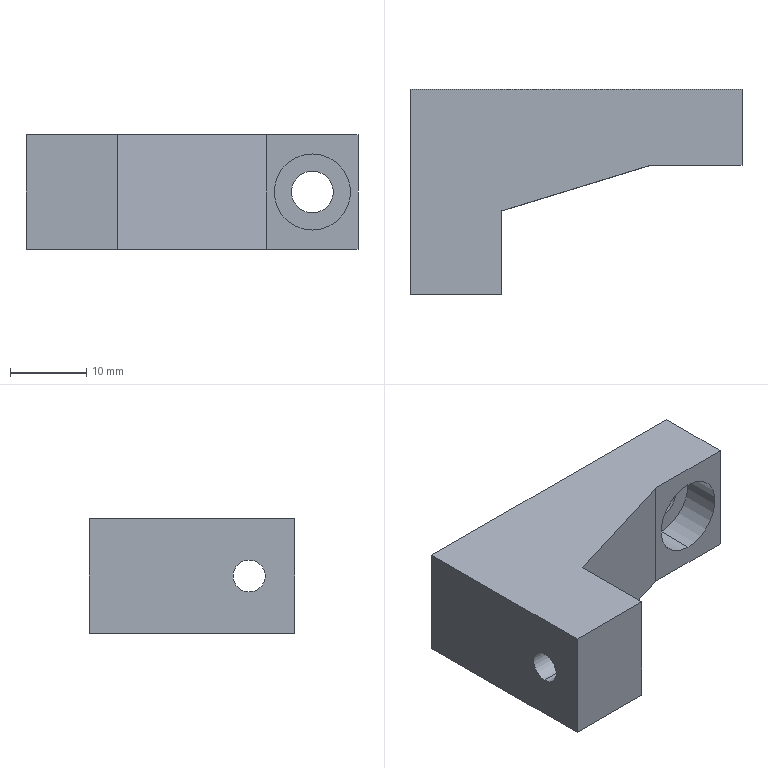Part | NX | features BREP 1 | 1 solid | 16 faces | box 43.58 x 27 x 15 mm | volume 9800 mm3 | plane 10 | cylinder 6 | commonest cylinder face diameters 4.2 x2 5.5 x2 10 x2
STEP:
#1=CARTESIAN_POINT('',(-1048.919,61.885,12.5));
#2=VERTEX_POINT('',#1);
#3=CARTESIAN_POINT('',(-1048.919,61.885,2.5));
#4=VERTEX_POINT('',#3);
#5=CARTESIAN_POINT('',(-1048.919,61.885,7.5));
#6=DIRECTION('',(0.,-1.,0.));
#7=DIRECTION('',(0.,0.,-1.));
#8=AXIS2_PLACEMENT_3D('',#5,#6,#7);
#9=CIRCLE('',#8,5.);
#10=EDGE_CURVE('',#2,#4,#9,.T.);
#11=ORIENTED_EDGE('',*,*,#10,.F.);
#12=CARTESIAN_POINT('',(-1048.919,56.885,12.5));
#13=VERTEX_POINT('',#12);
#14=CARTESIAN_POINT('',(-1048.919,56.885,12.5));
#15=DIRECTION('',(0.,-1.,0.));
#16=VECTOR('',#15,1000.);
#17=LINE('',#14,#16);
#18=EDGE_CURVE('',#2,#13,#17,.T.);
#19=ORIENTED_EDGE('',*,*,#18,.T.);
#20=CARTESIAN_POINT('',(-1048.919,56.885,2.5));
#21=VERTEX_POINT('',#20);
#22=CARTESIAN_POINT('',(-1048.919,56.885,7.5));
#23=DIRECTION('',(0.,-1.,0.));
#24=DIRECTION('',(0.,0.,-1.));
#25=AXIS2_PLACEMENT_3D('',#22,#23,#24);
#26=CIRCLE('',#25,5.);
#27=EDGE_CURVE('',#13,#21,#26,.T.);
#28=ORIENTED_EDGE('',*,*,#27,.T.);
#29=CARTESIAN_POINT('',(-1048.919,56.885,2.5));
#30=DIRECTION('',(0.,-1.,0.));
#31=VECTOR('',#30,1000.);
#32=LINE('',#29,#31);
#33=EDGE_CURVE('',#4,#21,#32,.T.);
#34=ORIENTED_EDGE('',*,*,#33,.F.);
#35=EDGE_LOOP('',(#11,#19,#28,#34));
#36=FACE_BOUND('',#35,.T.);
#37=CARTESIAN_POINT('',(-1048.919,56.885,7.5));
#38=DIRECTION('',(0.,-1.,0.));
#39=DIRECTION('',(0.,0.,-1.));
#40=AXIS2_PLACEMENT_3D('',#37,#38,#39);
#41=CYLINDRICAL_SURFACE('',#40,5.);
#42=ADVANCED_FACE('',(#36),#41,.F.);
#43=CARTESIAN_POINT('',(-1048.919,66.885,10.25));
#44=VERTEX_POINT('',#43);
#45=CARTESIAN_POINT('',(-1048.919,66.885,4.75));
#46=VERTEX_POINT('',#45);
#47=CARTESIAN_POINT('',(-1048.919,66.885,7.5));
#48=DIRECTION('',(0.,-1.,0.));
#49=DIRECTION('',(0.,0.,-1.));
#50=AXIS2_PLACEMENT_3D('',#47,#48,#49);
#51=CIRCLE('',#50,2.75);
#52=EDGE_CURVE('',#44,#46,#51,.T.);
#53=ORIENTED_EDGE('',*,*,#52,.F.);
#54=CARTESIAN_POINT('',(-1048.919,61.885,10.25));
#55=VERTEX_POINT('',#54);
#56=CARTESIAN_POINT('',(-1048.919,56.885,10.25));
#57=DIRECTION('',(0.,-1.,0.));
#58=VECTOR('',#57,1000.);
#59=LINE('',#56,#58);
#60=EDGE_CURVE('',#44,#55,#59,.T.);
#61=ORIENTED_EDGE('',*,*,#60,.T.);
#62=CARTESIAN_POINT('',(-1048.919,61.885,4.75));
#63=VERTEX_POINT('',#62);
#64=CARTESIAN_POINT('',(-1048.919,61.885,7.5));
#65=DIRECTION('',(0.,-1.,0.));
#66=DIRECTION('',(0.,0.,-1.));
#67=AXIS2_PLACEMENT_3D('',#64,#65,#66);
#68=CIRCLE('',#67,2.75);
#69=EDGE_CURVE('',#55,#63,#68,.T.);
#70=ORIENTED_EDGE('',*,*,#69,.T.);
#71=CARTESIAN_POINT('',(-1048.919,56.885,4.75));
#72=DIRECTION('',(0.,-1.,0.));
#73=VECTOR('',#72,1000.);
#74=LINE('',#71,#73);
#75=EDGE_CURVE('',#46,#63,#74,.T.);
#76=ORIENTED_EDGE('',*,*,#75,.F.);
#77=EDGE_LOOP('',(#53,#61,#70,#76));
#78=FACE_BOUND('',#77,.T.);
#79=CARTESIAN_POINT('',(-1048.919,56.885,7.5));
#80=DIRECTION('',(0.,-1.,0.));
#81=DIRECTION('',(0.,0.,-1.));
#82=AXIS2_PLACEMENT_3D('',#79,#80,#81);
#83=CYLINDRICAL_SURFACE('',#82,2.75);
#84=ADVANCED_FACE('',(#78),#83,.F.);
#85=CARTESIAN_POINT('',(-1074.5,45.885,5.4));
#86=VERTEX_POINT('',#85);
#87=CARTESIAN_POINT('',(-1074.5,45.885,9.6));
#88=VERTEX_POINT('',#87);
#89=CARTESIAN_POINT('',(-1074.5,45.885,7.5));
#90=DIRECTION('',(-1.,0.,0.));
#91=DIRECTION('',(0.,0.,1.));
#92=AXIS2_PLACEMENT_3D('',#89,#90,#91);
#93=CIRCLE('',#92,2.1);
#94=EDGE_CURVE('',#86,#88,#93,.T.);
#95=ORIENTED_EDGE('',*,*,#94,.F.);
#96=CARTESIAN_POINT('',(-1086.5,45.885,5.4));
#97=VERTEX_POINT('',#96);
#98=CARTESIAN_POINT('',(-1086.5,45.885,5.4));
#99=DIRECTION('',(-1.,0.,0.));
#100=VECTOR('',#99,1000.);
#101=LINE('',#98,#100);
#102=EDGE_CURVE('',#97,#86,#101,.F.);
#103=ORIENTED_EDGE('',*,*,#102,.F.);
#104=CARTESIAN_POINT('',(-1086.5,45.885,9.6));
#105=VERTEX_POINT('',#104);
#106=CARTESIAN_POINT('',(-1086.5,45.885,7.5));
#107=DIRECTION('',(-1.,0.,0.));
#108=DIRECTION('',(0.,0.,1.));
#109=AXIS2_PLACEMENT_3D('',#106,#107,#108);
#110=CIRCLE('',#109,2.1);
#111=EDGE_CURVE('',#97,#105,#110,.T.);
#112=ORIENTED_EDGE('',*,*,#111,.T.);
#113=CARTESIAN_POINT('',(-1086.5,45.885,9.6));
#114=DIRECTION('',(-1.,0.,0.));
#115=VECTOR('',#114,1000.);
#116=LINE('',#113,#115);
#117=EDGE_CURVE('',#105,#88,#116,.F.);
#118=ORIENTED_EDGE('',*,*,#117,.T.);
#119=EDGE_LOOP('',(#95,#103,#112,#118));
#120=FACE_BOUND('',#119,.T.);
#121=CARTESIAN_POINT('',(-1086.5,45.885,7.5));
#122=DIRECTION('',(-1.,0.,0.));
#123=DIRECTION('',(0.,0.,1.));
#124=AXIS2_PLACEMENT_3D('',#121,#122,#123);
#125=CYLINDRICAL_SURFACE('',#124,2.1);
#126=ADVANCED_FACE('',(#120),#125,.F.);
#127=CARTESIAN_POINT('',(-1086.5,39.885,0.));
#128=VERTEX_POINT('',#127);
#129=CARTESIAN_POINT('',(-1074.5,39.885,0.));
#130=VERTEX_POINT('',#129);
#131=CARTESIAN_POINT('',(-1086.5,39.885,0.));
#132=DIRECTION('',(1.,0.,0.));
#133=VECTOR('',#132,1000.);
#134=LINE('',#131,#133);
#135=EDGE_CURVE('',#128,#130,#134,.T.);
#136=ORIENTED_EDGE('',*,*,#135,.T.);
#137=CARTESIAN_POINT('',(-1074.5,39.885,15.));
#138=VERTEX_POINT('',#137);
#139=CARTESIAN_POINT('',(-1074.5,39.885,15.));
#140=DIRECTION('',(0.,0.,-1.));
#141=VECTOR('',#140,1000.);
#142=LINE('',#139,#141);
#143=EDGE_CURVE('',#138,#130,#142,.T.);
#144=ORIENTED_EDGE('',*,*,#143,.F.);
#145=CARTESIAN_POINT('',(-1086.5,39.885,15.));
#146=VERTEX_POINT('',#145);
#147=CARTESIAN_POINT('',(-1086.5,39.885,15.));
#148=DIRECTION('',(1.,0.,0.));
#149=VECTOR('',#148,1000.);
#150=LINE('',#147,#149);
#151=EDGE_CURVE('',#146,#138,#150,.T.);
#152=ORIENTED_EDGE('',*,*,#151,.F.);
#153=CARTESIAN_POINT('',(-1086.5,39.885,15.));
#154=DIRECTION('',(0.,0.,-1.));
#155=VECTOR('',#154,1000.);
#156=LINE('',#153,#155);
#157=EDGE_CURVE('',#146,#128,#156,.T.);
#158=ORIENTED_EDGE('',*,*,#157,.T.);
#159=EDGE_LOOP('',(#136,#144,#152,#158));
#160=FACE_BOUND('',#159,.T.);
#161=CARTESIAN_POINT('',(-1086.5,39.885,15.));
#162=DIRECTION('',(0.,1.,0.));
#163=DIRECTION('',(1.,0.,0.));
#164=AXIS2_PLACEMENT_3D('',#161,#162,#163);
#165=PLANE('',#164);
#166=ADVANCED_FACE('',(#160),#165,.F.);
#167=CARTESIAN_POINT('',(-1074.5,50.885,0.));
#168=VERTEX_POINT('',#167);
#169=CARTESIAN_POINT('',(-1074.5,39.885,0.));
#170=DIRECTION('',(0.,1.,0.));
#171=VECTOR('',#170,1000.);
#172=LINE('',#169,#171);
#173=EDGE_CURVE('',#130,#168,#172,.T.);
#174=ORIENTED_EDGE('',*,*,#173,.T.);
#175=CARTESIAN_POINT('',(-1074.5,50.885,15.));
#176=VERTEX_POINT('',#175);
#177=CARTESIAN_POINT('',(-1074.5,50.885,15.));
#178=DIRECTION('',(0.,0.,-1.));
#179=VECTOR('',#178,1000.);
#180=LINE('',#177,#179);
#181=EDGE_CURVE('',#176,#168,#180,.T.);
#182=ORIENTED_EDGE('',*,*,#181,.F.);
#183=CARTESIAN_POINT('',(-1074.5,39.885,15.));
#184=DIRECTION('',(0.,1.,0.));
#185=VECTOR('',#184,1000.);
#186=LINE('',#183,#185);
#187=EDGE_CURVE('',#138,#176,#186,.T.);
#188=ORIENTED_EDGE('',*,*,#187,.F.);
#189=ORIENTED_EDGE('',*,*,#143,.T.);
#190=EDGE_LOOP('',(#174,#182,#188,#189));
#191=FACE_BOUND('',#190,.T.);
#192=CARTESIAN_POINT('',(-1074.5,45.885,7.5));
#193=DIRECTION('',(-1.,0.,0.));
#194=DIRECTION('',(0.,0.,1.));
#195=AXIS2_PLACEMENT_3D('',#192,#193,#194);
#196=CIRCLE('',#195,2.1);
#197=EDGE_CURVE('',#88,#86,#196,.T.);
#198=ORIENTED_EDGE('',*,*,#197,.T.);
#199=ORIENTED_EDGE('',*,*,#94,.T.);
#200=EDGE_LOOP('',(#198,#199));
#201=FACE_BOUND('',#200,.T.);
#202=CARTESIAN_POINT('',(-1074.5,39.885,15.));
#203=DIRECTION('',(-1.,0.,0.));
#204=DIRECTION('',(0.,0.,1.));
#205=AXIS2_PLACEMENT_3D('',#202,#203,#204);
#206=PLANE('',#205);
#207=ADVANCED_FACE('',(#191,#201),#206,.F.);
#208=CARTESIAN_POINT('',(-1054.919,56.885,0.));
#209=VERTEX_POINT('',#208);
#210=CARTESIAN_POINT('',(-1074.5,50.885,0.));
#211=DIRECTION('',(0.9561,0.293,0.));
#212=VECTOR('',#211,1000.);
#213=LINE('',#210,#212);
#214=EDGE_CURVE('',#168,#209,#213,.T.);
#215=ORIENTED_EDGE('',*,*,#214,.T.);
#216=CARTESIAN_POINT('',(-1054.919,56.885,15.));
#217=VERTEX_POINT('',#216);
#218=CARTESIAN_POINT('',(-1054.919,56.885,15.));
#219=DIRECTION('',(0.,0.,-1.));
#220=VECTOR('',#219,1000.);
#221=LINE('',#218,#220);
#222=EDGE_CURVE('',#217,#209,#221,.T.);
#223=ORIENTED_EDGE('',*,*,#222,.F.);
#224=CARTESIAN_POINT('',(-1074.5,50.885,15.));
#225=DIRECTION('',(0.9561,0.293,0.));
#226=VECTOR('',#225,1000.);
#227=LINE('',#224,#226);
#228=EDGE_CURVE('',#176,#217,#227,.T.);
#229=ORIENTED_EDGE('',*,*,#228,.F.);
#230=ORIENTED_EDGE('',*,*,#181,.T.);
#231=EDGE_LOOP('',(#215,#223,#229,#230));
#232=FACE_BOUND('',#231,.T.);
#233=CARTESIAN_POINT('',(-1074.5,50.885,15.));
#234=DIRECTION('',(-0.293,0.9561,0.));
#235=DIRECTION('',(0.,0.,1.));
#236=AXIS2_PLACEMENT_3D('',#233,#234,#235);
#237=PLANE('',#236);
#238=ADVANCED_FACE('',(#232),#237,.F.);
#239=CARTESIAN_POINT('',(-1042.919,56.885,0.));
#240=VERTEX_POINT('',#239);
#241=CARTESIAN_POINT('',(-1054.919,56.885,0.));
#242=DIRECTION('',(1.,0.,0.));
#243=VECTOR('',#242,1000.);
#244=LINE('',#241,#243);
#245=EDGE_CURVE('',#209,#240,#244,.T.);
#246=ORIENTED_EDGE('',*,*,#245,.T.);
#247=CARTESIAN_POINT('',(-1042.919,56.885,15.));
#248=VERTEX_POINT('',#247);
#249=CARTESIAN_POINT('',(-1042.919,56.885,15.));
#250=DIRECTION('',(0.,0.,-1.));
#251=VECTOR('',#250,1000.);
#252=LINE('',#249,#251);
#253=EDGE_CURVE('',#248,#240,#252,.T.);
#254=ORIENTED_EDGE('',*,*,#253,.F.);
#255=CARTESIAN_POINT('',(-1054.919,56.885,15.));
#256=DIRECTION('',(1.,0.,0.));
#257=VECTOR('',#256,1000.);
#258=LINE('',#255,#257);
#259=EDGE_CURVE('',#217,#248,#258,.T.);
#260=ORIENTED_EDGE('',*,*,#259,.F.);
#261=ORIENTED_EDGE('',*,*,#222,.T.);
#262=EDGE_LOOP('',(#246,#254,#260,#261));
#263=FACE_BOUND('',#262,.T.);
#264=CARTESIAN_POINT('',(-1048.919,56.885,7.5));
#265=DIRECTION('',(0.,-1.,0.));
#266=DIRECTION('',(0.,0.,-1.));
#267=AXIS2_PLACEMENT_3D('',#264,#265,#266);
#268=CIRCLE('',#267,5.);
#269=EDGE_CURVE('',#21,#13,#268,.T.);
#270=ORIENTED_EDGE('',*,*,#269,.F.);
#271=ORIENTED_EDGE('',*,*,#27,.F.);
#272=EDGE_LOOP('',(#270,#271));
#273=FACE_BOUND('',#272,.T.);
#274=CARTESIAN_POINT('',(-1054.919,56.885,15.));
#275=DIRECTION('',(0.,1.,0.));
#276=DIRECTION('',(1.,0.,0.));
#277=AXIS2_PLACEMENT_3D('',#274,#275,#276);
#278=PLANE('',#277);
#279=ADVANCED_FACE('',(#263,#273),#278,.F.);
#280=CARTESIAN_POINT('',(-1042.919,66.885,0.));
#281=VERTEX_POINT('',#280);
#282=CARTESIAN_POINT('',(-1042.919,56.885,0.));
#283=DIRECTION('',(0.,1.,0.));
#284=VECTOR('',#283,1000.);
#285=LINE('',#282,#284);
#286=EDGE_CURVE('',#240,#281,#285,.T.);
#287=ORIENTED_EDGE('',*,*,#286,.T.);
#288=CARTESIAN_POINT('',(-1042.919,66.885,15.));
#289=VERTEX_POINT('',#288);
#290=CARTESIAN_POINT('',(-1042.919,66.885,15.));
#291=DIRECTION('',(0.,0.,-1.));
#292=VECTOR('',#291,1000.);
#293=LINE('',#290,#292);
#294=EDGE_CURVE('',#289,#281,#293,.T.);
#295=ORIENTED_EDGE('',*,*,#294,.F.);
#296=CARTESIAN_POINT('',(-1042.919,56.885,15.));
#297=DIRECTION('',(0.,1.,0.));
#298=VECTOR('',#297,1000.);
#299=LINE('',#296,#298);
#300=EDGE_CURVE('',#248,#289,#299,.T.);
#301=ORIENTED_EDGE('',*,*,#300,.F.);
#302=ORIENTED_EDGE('',*,*,#253,.T.);
#303=EDGE_LOOP('',(#287,#295,#301,#302));
#304=FACE_BOUND('',#303,.T.);
#305=CARTESIAN_POINT('',(-1042.919,56.885,15.));
#306=DIRECTION('',(-1.,0.,0.));
#307=DIRECTION('',(0.,0.,1.));
#308=AXIS2_PLACEMENT_3D('',#305,#306,#307);
#309=PLANE('',#308);
#310=ADVANCED_FACE('',(#304),#309,.F.);
#311=CARTESIAN_POINT('',(-1086.5,66.885,0.));
#312=VERTEX_POINT('',#311);
#313=CARTESIAN_POINT('',(-1042.919,66.885,0.));
#314=DIRECTION('',(-1.,0.,0.));
#315=VECTOR('',#314,1000.);
#316=LINE('',#313,#315);
#317=EDGE_CURVE('',#281,#312,#316,.T.);
#318=ORIENTED_EDGE('',*,*,#317,.T.);
#319=CARTESIAN_POINT('',(-1086.5,66.885,15.));
#320=VERTEX_POINT('',#319);
#321=CARTESIAN_POINT('',(-1086.5,66.885,15.));
#322=DIRECTION('',(0.,0.,-1.));
#323=VECTOR('',#322,1000.);
#324=LINE('',#321,#323);
#325=EDGE_CURVE('',#320,#312,#324,.T.);
#326=ORIENTED_EDGE('',*,*,#325,.F.);
#327=CARTESIAN_POINT('',(-1042.919,66.885,15.));
#328=DIRECTION('',(-1.,0.,0.));
#329=VECTOR('',#328,1000.);
#330=LINE('',#327,#329);
#331=EDGE_CURVE('',#289,#320,#330,.T.);
#332=ORIENTED_EDGE('',*,*,#331,.F.);
#333=ORIENTED_EDGE('',*,*,#294,.T.);
#334=EDGE_LOOP('',(#318,#326,#332,#333));
#335=FACE_BOUND('',#334,.T.);
#336=CARTESIAN_POINT('',(-1048.919,66.885,7.5));
#337=DIRECTION('',(0.,-1.,0.));
#338=DIRECTION('',(0.,0.,-1.));
#339=AXIS2_PLACEMENT_3D('',#336,#337,#338);
#340=CIRCLE('',#339,2.75);
#341=EDGE_CURVE('',#46,#44,#340,.T.);
#342=ORIENTED_EDGE('',*,*,#341,.T.);
#343=ORIENTED_EDGE('',*,*,#52,.T.);
#344=EDGE_LOOP('',(#342,#343));
#345=FACE_BOUND('',#344,.T.);
#346=CARTESIAN_POINT('',(-1042.919,66.885,15.));
#347=DIRECTION('',(0.,-1.,0.));
#348=DIRECTION('',(0.,0.,-1.));
#349=AXIS2_PLACEMENT_3D('',#346,#347,#348);
#350=PLANE('',#349);
#351=ADVANCED_FACE('',(#335,#345),#350,.F.);
#352=CARTESIAN_POINT('',(-1086.5,66.885,0.));
#353=DIRECTION('',(0.,-1.,0.));
#354=VECTOR('',#353,1000.);
#355=LINE('',#352,#354);
#356=EDGE_CURVE('',#312,#128,#355,.T.);
#357=ORIENTED_EDGE('',*,*,#356,.T.);
#358=ORIENTED_EDGE('',*,*,#157,.F.);
#359=CARTESIAN_POINT('',(-1086.5,66.885,15.));
#360=DIRECTION('',(0.,-1.,0.));
#361=VECTOR('',#360,1000.);
#362=LINE('',#359,#361);
#363=EDGE_CURVE('',#320,#146,#362,.T.);
#364=ORIENTED_EDGE('',*,*,#363,.F.);
#365=ORIENTED_EDGE('',*,*,#325,.T.);
#366=EDGE_LOOP('',(#357,#358,#364,#365));
#367=FACE_BOUND('',#366,.T.);
#368=CARTESIAN_POINT('',(-1086.5,45.885,7.5));
#369=DIRECTION('',(-1.,0.,0.));
#370=DIRECTION('',(0.,0.,1.));
#371=AXIS2_PLACEMENT_3D('',#368,#369,#370);
#372=CIRCLE('',#371,2.1);
#373=EDGE_CURVE('',#105,#97,#372,.T.);
#374=ORIENTED_EDGE('',*,*,#373,.F.);
#375=ORIENTED_EDGE('',*,*,#111,.F.);
#376=EDGE_LOOP('',(#374,#375));
#377=FACE_BOUND('',#376,.T.);
#378=CARTESIAN_POINT('',(-1086.5,66.885,15.));
#379=DIRECTION('',(1.,0.,0.));
#380=DIRECTION('',(0.,1.,0.));
#381=AXIS2_PLACEMENT_3D('',#378,#379,#380);
#382=PLANE('',#381);
#383=ADVANCED_FACE('',(#367,#377),#382,.F.);
#384=ORIENTED_EDGE('',*,*,#151,.T.);
#385=ORIENTED_EDGE('',*,*,#187,.T.);
#386=ORIENTED_EDGE('',*,*,#228,.T.);
#387=ORIENTED_EDGE('',*,*,#259,.T.);
#388=ORIENTED_EDGE('',*,*,#300,.T.);
#389=ORIENTED_EDGE('',*,*,#331,.T.);
#390=ORIENTED_EDGE('',*,*,#363,.T.);
#391=EDGE_LOOP('',(#384,#385,#386,#387,#388,#389,#390));
#392=FACE_BOUND('',#391,.T.);
#393=CARTESIAN_POINT('',(-1074.5,39.885,15.));
#394=DIRECTION('',(0.,0.,1.));
#395=DIRECTION('',(1.,0.,0.));
#396=AXIS2_PLACEMENT_3D('',#393,#394,#395);
#397=PLANE('',#396);
#398=ADVANCED_FACE('',(#392),#397,.T.);
#399=ORIENTED_EDGE('',*,*,#135,.F.);
#400=ORIENTED_EDGE('',*,*,#356,.F.);
#401=ORIENTED_EDGE('',*,*,#317,.F.);
#402=ORIENTED_EDGE('',*,*,#286,.F.);
#403=ORIENTED_EDGE('',*,*,#245,.F.);
#404=ORIENTED_EDGE('',*,*,#214,.F.);
#405=ORIENTED_EDGE('',*,*,#173,.F.);
#406=EDGE_LOOP('',(#399,#400,#401,#402,#403,#404,#405));
#407=FACE_BOUND('',#406,.T.);
#408=CARTESIAN_POINT('',(-1074.5,39.885,0.));
#409=DIRECTION('',(0.,0.,1.));
#410=DIRECTION('',(1.,0.,0.));
#411=AXIS2_PLACEMENT_3D('',#408,#409,#410);
#412=PLANE('',#411);
#413=ADVANCED_FACE('',(#407),#412,.F.);
#414=ORIENTED_EDGE('',*,*,#102,.T.);
#415=ORIENTED_EDGE('',*,*,#197,.F.);
#416=ORIENTED_EDGE('',*,*,#117,.F.);
#417=ORIENTED_EDGE('',*,*,#373,.T.);
#418=EDGE_LOOP('',(#414,#415,#416,#417));
#419=FACE_BOUND('',#418,.T.);
#420=CARTESIAN_POINT('',(-1086.5,45.885,7.5));
#421=DIRECTION('',(-1.,0.,0.));
#422=DIRECTION('',(0.,0.,1.));
#423=AXIS2_PLACEMENT_3D('',#420,#421,#422);
#424=CYLINDRICAL_SURFACE('',#423,2.1);
#425=ADVANCED_FACE('',(#419),#424,.F.);
#426=ORIENTED_EDGE('',*,*,#60,.F.);
#427=ORIENTED_EDGE('',*,*,#341,.F.);
#428=ORIENTED_EDGE('',*,*,#75,.T.);
#429=CARTESIAN_POINT('',(-1048.919,61.885,7.5));
#430=DIRECTION('',(0.,-1.,0.));
#431=DIRECTION('',(0.,0.,-1.));
#432=AXIS2_PLACEMENT_3D('',#429,#430,#431);
#433=CIRCLE('',#432,2.75);
#434=EDGE_CURVE('',#63,#55,#433,.T.);
#435=ORIENTED_EDGE('',*,*,#434,.T.);
#436=EDGE_LOOP('',(#426,#427,#428,#435));
#437=FACE_BOUND('',#436,.T.);
#438=CARTESIAN_POINT('',(-1048.919,56.885,7.5));
#439=DIRECTION('',(0.,-1.,0.));
#440=DIRECTION('',(0.,0.,-1.));
#441=AXIS2_PLACEMENT_3D('',#438,#439,#440);
#442=CYLINDRICAL_SURFACE('',#441,2.75);
#443=ADVANCED_FACE('',(#437),#442,.F.);
#444=CARTESIAN_POINT('',(-1048.919,61.885,7.5));
#445=DIRECTION('',(0.,-1.,0.));
#446=DIRECTION('',(0.,0.,-1.));
#447=AXIS2_PLACEMENT_3D('',#444,#445,#446);
#448=CIRCLE('',#447,5.);
#449=EDGE_CURVE('',#4,#2,#448,.T.);
#450=ORIENTED_EDGE('',*,*,#449,.T.);
#451=ORIENTED_EDGE('',*,*,#10,.T.);
#452=EDGE_LOOP('',(#450,#451));
#453=FACE_BOUND('',#452,.T.);
#454=ORIENTED_EDGE('',*,*,#434,.F.);
#455=ORIENTED_EDGE('',*,*,#69,.F.);
#456=EDGE_LOOP('',(#454,#455));
#457=FACE_BOUND('',#456,.T.);
#458=CARTESIAN_POINT('',(-1046.169,61.885,7.5));
#459=DIRECTION('',(0.,1.,0.));
#460=DIRECTION('',(1.,0.,0.));
#461=AXIS2_PLACEMENT_3D('',#458,#459,#460);
#462=PLANE('',#461);
#463=ADVANCED_FACE('',(#453,#457),#462,.F.);
#464=ORIENTED_EDGE('',*,*,#18,.F.);
#465=ORIENTED_EDGE('',*,*,#449,.F.);
#466=ORIENTED_EDGE('',*,*,#33,.T.);
#467=ORIENTED_EDGE('',*,*,#269,.T.);
#468=EDGE_LOOP('',(#464,#465,#466,#467));
#469=FACE_BOUND('',#468,.T.);
#470=CARTESIAN_POINT('',(-1048.919,56.885,7.5));
#471=DIRECTION('',(0.,-1.,0.));
#472=DIRECTION('',(0.,0.,-1.));
#473=AXIS2_PLACEMENT_3D('',#470,#471,#472);
#474=CYLINDRICAL_SURFACE('',#473,5.);
#475=ADVANCED_FACE('',(#469),#474,.F.);
#476=CLOSED_SHELL('',(#42,#84,#126,#166,#207,#238,#279,#310,#351,#383,#398,#413,#425,#443,#463,#475));
#477=MANIFOLD_SOLID_BREP('',#476);
#478=(LENGTH_UNIT()NAMED_UNIT(*)SI_UNIT(.MILLI.,.METRE.));
#479=UNCERTAINTY_MEASURE_WITH_UNIT(LENGTH_MEASURE(0.00001),#478,'','');
#480=(NAMED_UNIT(*)PLANE_ANGLE_UNIT()SI_UNIT($,.RADIAN.));
#481=(NAMED_UNIT(*)SI_UNIT($,.STERADIAN.)SOLID_ANGLE_UNIT());
#482=(GEOMETRIC_REPRESENTATION_CONTEXT(3)GLOBAL_UNCERTAINTY_ASSIGNED_CONTEXT((#479))GLOBAL_UNIT_ASSIGNED_CONTEXT((#478,#480,#481))REPRESENTATION_CONTEXT('',''));
#483=ADVANCED_BREP_SHAPE_REPRESENTATION('',(#477),#482);